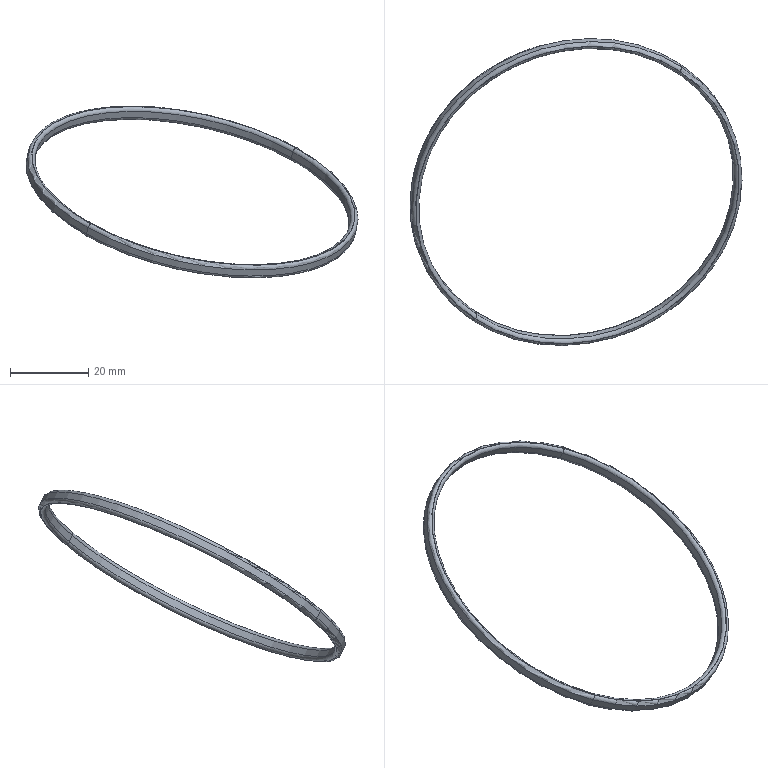Part | SolidWorks | features BaseBody 1 | 1 solid | 14 faces | box 84.752 x 78.463 x 43.87 mm | volume 1584 mm3 | torus 8 | cylinder 4 | plane 2 | commonest cylinder face diameters 82.4 x2 86.12 x2
STEP:
#1=CARTESIAN_POINT('',(1980.179,-187.025,950.905));
#2=VERTEX_POINT('',#1);
#3=CARTESIAN_POINT('',(1929.089,-248.825,931.919));
#4=VERTEX_POINT('',#3);
#5=CARTESIAN_POINT('',(1954.634,-217.925,941.412));
#6=DIRECTION('',(0.2015,-0.436,0.8771));
#7=DIRECTION('',(0.9077,0.4197,0.0001618));
#8=AXIS2_PLACEMENT_3D('',#5,#6,#7);
#9=CIRCLE('',#8,41.2);
#10=EDGE_CURVE('',#2,#4,#9,.T.);
#11=ORIENTED_EDGE('',*,*,#10,.F.);
#12=CARTESIAN_POINT('',(1980.539,-187.806,952.475));
#13=VERTEX_POINT('',#12);
#14=CARTESIAN_POINT('',(1980.359,-187.416,951.69));
#15=DIRECTION('',(0.2015,-0.436,0.8771));
#16=VECTOR('',#15,1000.);
#17=LINE('',#14,#16);
#18=EDGE_CURVE('',#2,#13,#17,.T.);
#19=ORIENTED_EDGE('',*,*,#18,.T.);
#20=CARTESIAN_POINT('',(1929.45,-249.605,933.489));
#21=VERTEX_POINT('',#20);
#22=CARTESIAN_POINT('',(1954.995,-218.706,942.982));
#23=DIRECTION('',(0.2015,-0.436,0.8771));
#24=DIRECTION('',(0.9077,0.4197,0.0001618));
#25=AXIS2_PLACEMENT_3D('',#22,#23,#24);
#26=CIRCLE('',#25,41.2);
#27=EDGE_CURVE('',#13,#21,#26,.T.);
#28=ORIENTED_EDGE('',*,*,#27,.T.);
#29=CARTESIAN_POINT('',(1929.27,-249.215,932.704));
#30=DIRECTION('',(-0.2015,0.436,-0.8771));
#31=VECTOR('',#30,1000.);
#32=LINE('',#29,#31);
#33=EDGE_CURVE('',#21,#4,#32,.T.);
#34=ORIENTED_EDGE('',*,*,#33,.T.);
#35=EDGE_LOOP('',(#11,#19,#28,#34));
#36=FACE_OUTER_BOUND('',#35,.T.);
#37=CARTESIAN_POINT('',(1954.814,-218.315,942.197));
#38=DIRECTION('',(0.2015,-0.436,0.8771));
#39=DIRECTION('',(-0.62,-0.75,-0.2304));
#40=AXIS2_PLACEMENT_3D('',#37,#38,#39);
#41=CYLINDRICAL_SURFACE('',#40,41.2);
#42=ADVANCED_FACE('',(#36),#41,.F.);
#43=CARTESIAN_POINT('',(1954.634,-217.925,941.412));
#44=DIRECTION('',(0.2015,-0.436,0.8771));
#45=DIRECTION('',(0.9077,0.4197,0.0001618));
#46=AXIS2_PLACEMENT_3D('',#43,#44,#45);
#47=CIRCLE('',#46,41.2);
#48=EDGE_CURVE('',#4,#2,#47,.T.);
#49=ORIENTED_EDGE('',*,*,#48,.F.);
#50=ORIENTED_EDGE('',*,*,#33,.F.);
#51=CARTESIAN_POINT('',(1954.995,-218.706,942.982));
#52=DIRECTION('',(0.2015,-0.436,0.8771));
#53=DIRECTION('',(0.9077,0.4197,0.0001618));
#54=AXIS2_PLACEMENT_3D('',#51,#52,#53);
#55=CIRCLE('',#54,41.2);
#56=EDGE_CURVE('',#21,#13,#55,.T.);
#57=ORIENTED_EDGE('',*,*,#56,.T.);
#58=ORIENTED_EDGE('',*,*,#18,.F.);
#59=EDGE_LOOP('',(#49,#50,#57,#58));
#60=FACE_OUTER_BOUND('',#59,.T.);
#61=CARTESIAN_POINT('',(1954.814,-218.315,942.197));
#62=DIRECTION('',(0.2015,-0.436,0.8771));
#63=DIRECTION('',(-0.62,-0.75,-0.2304));
#64=AXIS2_PLACEMENT_3D('',#61,#62,#63);
#65=CYLINDRICAL_SURFACE('',#64,41.2);
#66=ADVANCED_FACE('',(#60),#65,.F.);
#67=ORIENTED_EDGE('',*,*,#27,.F.);
#68=CARTESIAN_POINT('',(1981.279,-187.523,953.472));
#69=VERTEX_POINT('',#68);
#70=CARTESIAN_POINT('',(1981.097,-187.131,952.682));
#71=DIRECTION('',(0.7583,-0.4974,-0.4214));
#72=DIRECTION('',(0.62,0.75,0.2304));
#73=AXIS2_PLACEMENT_3D('',#70,#71,#72);
#74=CIRCLE('',#73,0.9);
#75=EDGE_CURVE('',#69,#13,#74,.T.);
#76=ORIENTED_EDGE('',*,*,#75,.F.);
#77=CARTESIAN_POINT('',(1929.073,-250.673,934.071));
#78=VERTEX_POINT('',#77);
#79=CARTESIAN_POINT('',(1955.176,-219.098,943.771));
#80=DIRECTION('',(0.2015,-0.436,0.8771));
#81=DIRECTION('',(0.9077,0.4197,0.0001618));
#82=AXIS2_PLACEMENT_3D('',#79,#80,#81);
#83=CIRCLE('',#82,42.1);
#84=EDGE_CURVE('',#69,#78,#83,.T.);
#85=ORIENTED_EDGE('',*,*,#84,.T.);
#86=CARTESIAN_POINT('',(1928.892,-250.28,933.281));
#87=DIRECTION('',(0.7583,-0.4974,-0.4214));
#88=DIRECTION('',(0.62,0.75,0.2304));
#89=AXIS2_PLACEMENT_3D('',#86,#87,#88);
#90=CIRCLE('',#89,0.9);
#91=EDGE_CURVE('',#21,#78,#90,.T.);
#92=ORIENTED_EDGE('',*,*,#91,.F.);
#93=EDGE_LOOP('',(#67,#76,#85,#92));
#94=FACE_OUTER_BOUND('',#93,.T.);
#95=CARTESIAN_POINT('',(1954.995,-218.706,942.982));
#96=DIRECTION('',(0.2015,-0.436,0.8771));
#97=DIRECTION('',(-0.62,-0.75,-0.2304));
#98=AXIS2_PLACEMENT_3D('',#95,#96,#97);
#99=TOROIDAL_SURFACE('',#98,42.1,0.9);
#100=ADVANCED_FACE('',(#94),#99,.T.);
#101=ORIENTED_EDGE('',*,*,#56,.F.);
#102=ORIENTED_EDGE('',*,*,#91,.T.);
#103=CARTESIAN_POINT('',(1955.176,-219.098,943.771));
#104=DIRECTION('',(0.2015,-0.436,0.8771));
#105=DIRECTION('',(0.9077,0.4197,0.0001618));
#106=AXIS2_PLACEMENT_3D('',#103,#104,#105);
#107=CIRCLE('',#106,42.1);
#108=EDGE_CURVE('',#78,#69,#107,.T.);
#109=ORIENTED_EDGE('',*,*,#108,.T.);
#110=ORIENTED_EDGE('',*,*,#75,.T.);
#111=EDGE_LOOP('',(#101,#102,#109,#110));
#112=FACE_OUTER_BOUND('',#111,.T.);
#113=CARTESIAN_POINT('',(1954.995,-218.706,942.982));
#114=DIRECTION('',(0.2015,-0.436,0.8771));
#115=DIRECTION('',(-0.62,-0.75,-0.2304));
#116=AXIS2_PLACEMENT_3D('',#113,#114,#115);
#117=TOROIDAL_SURFACE('',#116,42.1,0.9);
#118=ADVANCED_FACE('',(#112),#117,.T.);
#119=CARTESIAN_POINT('',(1981.316,-187.478,953.485));
#120=VERTEX_POINT('',#119);
#121=CARTESIAN_POINT('',(1929.036,-250.718,934.057));
#122=VERTEX_POINT('',#121);
#123=CARTESIAN_POINT('',(1955.176,-219.098,943.771));
#124=DIRECTION('',(0.2015,-0.436,0.8771));
#125=DIRECTION('',(0.9077,0.4197,0.0001618));
#126=AXIS2_PLACEMENT_3D('',#123,#124,#125);
#127=CIRCLE('',#126,42.16);
#128=EDGE_CURVE('',#120,#122,#127,.T.);
#129=ORIENTED_EDGE('',*,*,#128,.F.);
#130=CARTESIAN_POINT('',(1981.692,-186.411,952.903));
#131=VERTEX_POINT('',#130);
#132=CARTESIAN_POINT('',(1981.134,-187.086,952.696));
#133=DIRECTION('',(-0.7583,0.4974,0.4214));
#134=DIRECTION('',(0.62,0.75,0.2304));
#135=AXIS2_PLACEMENT_3D('',#132,#133,#134);
#136=CIRCLE('',#135,0.9);
#137=EDGE_CURVE('',#120,#131,#136,.T.);
#138=ORIENTED_EDGE('',*,*,#137,.T.);
#139=CARTESIAN_POINT('',(1928.297,-251.,933.06));
#140=VERTEX_POINT('',#139);
#141=CARTESIAN_POINT('',(1954.995,-218.706,942.982));
#142=DIRECTION('',(0.2015,-0.436,0.8771));
#143=DIRECTION('',(0.9077,0.4197,0.0001618));
#144=AXIS2_PLACEMENT_3D('',#141,#142,#143);
#145=CIRCLE('',#144,43.06);
#146=EDGE_CURVE('',#131,#140,#145,.T.);
#147=ORIENTED_EDGE('',*,*,#146,.T.);
#148=CARTESIAN_POINT('',(1928.855,-250.325,933.267));
#149=DIRECTION('',(-0.7583,0.4974,0.4214));
#150=DIRECTION('',(0.62,0.75,0.2304));
#151=AXIS2_PLACEMENT_3D('',#148,#149,#150);
#152=CIRCLE('',#151,0.9);
#153=EDGE_CURVE('',#140,#122,#152,.T.);
#154=ORIENTED_EDGE('',*,*,#153,.T.);
#155=EDGE_LOOP('',(#129,#138,#147,#154));
#156=FACE_OUTER_BOUND('',#155,.T.);
#157=CARTESIAN_POINT('',(1954.995,-218.706,942.982));
#158=DIRECTION('',(0.2015,-0.436,0.8771));
#159=DIRECTION('',(-0.62,-0.75,-0.2304));
#160=AXIS2_PLACEMENT_3D('',#157,#158,#159);
#161=TOROIDAL_SURFACE('',#160,42.16,0.9);
#162=ADVANCED_FACE('',(#156),#161,.T.);
#163=CARTESIAN_POINT('',(1955.176,-219.098,943.771));
#164=DIRECTION('',(0.2015,-0.436,0.8771));
#165=DIRECTION('',(0.9077,0.4197,0.0001618));
#166=AXIS2_PLACEMENT_3D('',#163,#164,#165);
#167=CIRCLE('',#166,42.16);
#168=EDGE_CURVE('',#122,#120,#167,.T.);
#169=ORIENTED_EDGE('',*,*,#168,.F.);
#170=ORIENTED_EDGE('',*,*,#153,.F.);
#171=CARTESIAN_POINT('',(1954.995,-218.706,942.982));
#172=DIRECTION('',(0.2015,-0.436,0.8771));
#173=DIRECTION('',(0.9077,0.4197,0.0001618));
#174=AXIS2_PLACEMENT_3D('',#171,#172,#173);
#175=CIRCLE('',#174,43.06);
#176=EDGE_CURVE('',#140,#131,#175,.T.);
#177=ORIENTED_EDGE('',*,*,#176,.T.);
#178=ORIENTED_EDGE('',*,*,#137,.F.);
#179=EDGE_LOOP('',(#169,#170,#177,#178));
#180=FACE_OUTER_BOUND('',#179,.T.);
#181=CARTESIAN_POINT('',(1954.995,-218.706,942.982));
#182=DIRECTION('',(0.2015,-0.436,0.8771));
#183=DIRECTION('',(-0.62,-0.75,-0.2304));
#184=AXIS2_PLACEMENT_3D('',#181,#182,#183);
#185=TOROIDAL_SURFACE('',#184,42.16,0.9);
#186=ADVANCED_FACE('',(#180),#185,.T.);
#187=ORIENTED_EDGE('',*,*,#146,.F.);
#188=CARTESIAN_POINT('',(1981.332,-185.63,951.333));
#189=VERTEX_POINT('',#188);
#190=CARTESIAN_POINT('',(1981.512,-186.021,952.118));
#191=DIRECTION('',(0.2015,-0.436,0.8771));
#192=VECTOR('',#191,1000.);
#193=LINE('',#190,#192);
#194=EDGE_CURVE('',#189,#131,#193,.T.);
#195=ORIENTED_EDGE('',*,*,#194,.F.);
#196=CARTESIAN_POINT('',(1927.936,-250.22,931.49));
#197=VERTEX_POINT('',#196);
#198=CARTESIAN_POINT('',(1954.634,-217.925,941.412));
#199=DIRECTION('',(0.2015,-0.436,0.8771));
#200=DIRECTION('',(0.9077,0.4197,0.0001618));
#201=AXIS2_PLACEMENT_3D('',#198,#199,#200);
#202=CIRCLE('',#201,43.06);
#203=EDGE_CURVE('',#189,#197,#202,.T.);
#204=ORIENTED_EDGE('',*,*,#203,.T.);
#205=CARTESIAN_POINT('',(1928.117,-250.61,932.275));
#206=DIRECTION('',(-0.2015,0.436,-0.8771));
#207=VECTOR('',#206,1000.);
#208=LINE('',#205,#207);
#209=EDGE_CURVE('',#140,#197,#208,.T.);
#210=ORIENTED_EDGE('',*,*,#209,.F.);
#211=EDGE_LOOP('',(#187,#195,#204,#210));
#212=FACE_OUTER_BOUND('',#211,.T.);
#213=CARTESIAN_POINT('',(1954.814,-218.315,942.197));
#214=DIRECTION('',(0.2015,-0.436,0.8771));
#215=DIRECTION('',(-0.62,-0.75,-0.2304));
#216=AXIS2_PLACEMENT_3D('',#213,#214,#215);
#217=CYLINDRICAL_SURFACE('',#216,43.06);
#218=ADVANCED_FACE('',(#212),#217,.T.);
#219=ORIENTED_EDGE('',*,*,#176,.F.);
#220=ORIENTED_EDGE('',*,*,#209,.T.);
#221=CARTESIAN_POINT('',(1954.634,-217.925,941.412));
#222=DIRECTION('',(0.2015,-0.436,0.8771));
#223=DIRECTION('',(0.9077,0.4197,0.0001618));
#224=AXIS2_PLACEMENT_3D('',#221,#222,#223);
#225=CIRCLE('',#224,43.06);
#226=EDGE_CURVE('',#197,#189,#225,.T.);
#227=ORIENTED_EDGE('',*,*,#226,.T.);
#228=ORIENTED_EDGE('',*,*,#194,.T.);
#229=EDGE_LOOP('',(#219,#220,#227,#228));
#230=FACE_OUTER_BOUND('',#229,.T.);
#231=CARTESIAN_POINT('',(1954.814,-218.315,942.197));
#232=DIRECTION('',(0.2015,-0.436,0.8771));
#233=DIRECTION('',(-0.62,-0.75,-0.2304));
#234=AXIS2_PLACEMENT_3D('',#231,#232,#233);
#235=CYLINDRICAL_SURFACE('',#234,43.06);
#236=ADVANCED_FACE('',(#230),#235,.T.);
#237=ORIENTED_EDGE('',*,*,#203,.F.);
#238=CARTESIAN_POINT('',(1980.592,-185.913,950.337));
#239=VERTEX_POINT('',#238);
#240=CARTESIAN_POINT('',(1980.774,-186.305,951.126));
#241=DIRECTION('',(0.7583,-0.4974,-0.4214));
#242=DIRECTION('',(0.62,0.75,0.2304));
#243=AXIS2_PLACEMENT_3D('',#240,#241,#242);
#244=CIRCLE('',#243,0.9);
#245=EDGE_CURVE('',#239,#189,#244,.T.);
#246=ORIENTED_EDGE('',*,*,#245,.F.);
#247=CARTESIAN_POINT('',(1928.313,-249.153,930.908));
#248=VERTEX_POINT('',#247);
#249=CARTESIAN_POINT('',(1954.453,-217.533,940.622));
#250=DIRECTION('',(0.2015,-0.436,0.8771));
#251=DIRECTION('',(0.9077,0.4197,0.0001618));
#252=AXIS2_PLACEMENT_3D('',#249,#250,#251);
#253=CIRCLE('',#252,42.16);
#254=EDGE_CURVE('',#239,#248,#253,.T.);
#255=ORIENTED_EDGE('',*,*,#254,.T.);
#256=CARTESIAN_POINT('',(1928.494,-249.545,931.697));
#257=DIRECTION('',(0.7583,-0.4974,-0.4214));
#258=DIRECTION('',(0.62,0.75,0.2304));
#259=AXIS2_PLACEMENT_3D('',#256,#257,#258);
#260=CIRCLE('',#259,0.9);
#261=EDGE_CURVE('',#197,#248,#260,.T.);
#262=ORIENTED_EDGE('',*,*,#261,.F.);
#263=EDGE_LOOP('',(#237,#246,#255,#262));
#264=FACE_OUTER_BOUND('',#263,.T.);
#265=CARTESIAN_POINT('',(1954.634,-217.925,941.412));
#266=DIRECTION('',(0.2015,-0.436,0.8771));
#267=DIRECTION('',(-0.62,-0.75,-0.2304));
#268=AXIS2_PLACEMENT_3D('',#265,#266,#267);
#269=TOROIDAL_SURFACE('',#268,42.16,0.9);
#270=ADVANCED_FACE('',(#264),#269,.T.);
#271=ORIENTED_EDGE('',*,*,#226,.F.);
#272=ORIENTED_EDGE('',*,*,#261,.T.);
#273=CARTESIAN_POINT('',(1954.453,-217.533,940.622));
#274=DIRECTION('',(0.2015,-0.436,0.8771));
#275=DIRECTION('',(0.9077,0.4197,0.0001618));
#276=AXIS2_PLACEMENT_3D('',#273,#274,#275);
#277=CIRCLE('',#276,42.16);
#278=EDGE_CURVE('',#248,#239,#277,.T.);
#279=ORIENTED_EDGE('',*,*,#278,.T.);
#280=ORIENTED_EDGE('',*,*,#245,.T.);
#281=EDGE_LOOP('',(#271,#272,#279,#280));
#282=FACE_OUTER_BOUND('',#281,.T.);
#283=CARTESIAN_POINT('',(1954.634,-217.925,941.412));
#284=DIRECTION('',(0.2015,-0.436,0.8771));
#285=DIRECTION('',(-0.62,-0.75,-0.2304));
#286=AXIS2_PLACEMENT_3D('',#283,#284,#285);
#287=TOROIDAL_SURFACE('',#286,42.16,0.9);
#288=ADVANCED_FACE('',(#282),#287,.T.);
#289=CARTESIAN_POINT('',(1980.555,-185.958,950.323));
#290=VERTEX_POINT('',#289);
#291=CARTESIAN_POINT('',(1928.35,-249.108,930.922));
#292=VERTEX_POINT('',#291);
#293=CARTESIAN_POINT('',(1954.453,-217.533,940.622));
#294=DIRECTION('',(0.2015,-0.436,0.8771));
#295=DIRECTION('',(0.9077,0.4197,0.0001618));
#296=AXIS2_PLACEMENT_3D('',#293,#294,#295);
#297=CIRCLE('',#296,42.1);
#298=EDGE_CURVE('',#290,#292,#297,.T.);
#299=ORIENTED_EDGE('',*,*,#298,.F.);
#300=CARTESIAN_POINT('',(1980.737,-186.35,951.112));
#301=DIRECTION('',(-0.7583,0.4974,0.4214));
#302=DIRECTION('',(0.62,0.75,0.2304));
#303=AXIS2_PLACEMENT_3D('',#300,#301,#302);
#304=CIRCLE('',#303,0.9);
#305=EDGE_CURVE('',#290,#2,#304,.T.);
#306=ORIENTED_EDGE('',*,*,#305,.T.);
#307=ORIENTED_EDGE('',*,*,#10,.T.);
#308=CARTESIAN_POINT('',(1928.531,-249.5,931.711));
#309=DIRECTION('',(-0.7583,0.4974,0.4214));
#310=DIRECTION('',(0.62,0.75,0.2304));
#311=AXIS2_PLACEMENT_3D('',#308,#309,#310);
#312=CIRCLE('',#311,0.9);
#313=EDGE_CURVE('',#4,#292,#312,.T.);
#314=ORIENTED_EDGE('',*,*,#313,.T.);
#315=EDGE_LOOP('',(#299,#306,#307,#314));
#316=FACE_OUTER_BOUND('',#315,.T.);
#317=CARTESIAN_POINT('',(1954.634,-217.925,941.412));
#318=DIRECTION('',(0.2015,-0.436,0.8771));
#319=DIRECTION('',(-0.62,-0.75,-0.2304));
#320=AXIS2_PLACEMENT_3D('',#317,#318,#319);
#321=TOROIDAL_SURFACE('',#320,42.1,0.9);
#322=ADVANCED_FACE('',(#316),#321,.T.);
#323=CARTESIAN_POINT('',(1954.453,-217.533,940.622));
#324=DIRECTION('',(0.2015,-0.436,0.8771));
#325=DIRECTION('',(0.9077,0.4197,0.0001618));
#326=AXIS2_PLACEMENT_3D('',#323,#324,#325);
#327=CIRCLE('',#326,42.1);
#328=EDGE_CURVE('',#292,#290,#327,.T.);
#329=ORIENTED_EDGE('',*,*,#328,.F.);
#330=ORIENTED_EDGE('',*,*,#313,.F.);
#331=ORIENTED_EDGE('',*,*,#48,.T.);
#332=ORIENTED_EDGE('',*,*,#305,.F.);
#333=EDGE_LOOP('',(#329,#330,#331,#332));
#334=FACE_OUTER_BOUND('',#333,.T.);
#335=CARTESIAN_POINT('',(1954.634,-217.925,941.412));
#336=DIRECTION('',(0.2015,-0.436,0.8771));
#337=DIRECTION('',(-0.62,-0.75,-0.2304));
#338=AXIS2_PLACEMENT_3D('',#335,#336,#337);
#339=TOROIDAL_SURFACE('',#338,42.1,0.9);
#340=ADVANCED_FACE('',(#334),#339,.T.);
#341=ORIENTED_EDGE('',*,*,#168,.T.);
#342=ORIENTED_EDGE('',*,*,#128,.T.);
#343=EDGE_LOOP('',(#341,#342));
#344=FACE_OUTER_BOUND('',#343,.T.);
#345=ORIENTED_EDGE('',*,*,#84,.F.);
#346=ORIENTED_EDGE('',*,*,#108,.F.);
#347=EDGE_LOOP('',(#345,#346));
#348=FACE_BOUND('',#347,.T.);
#349=CARTESIAN_POINT('',(1993.388,-201.428,943.778));
#350=DIRECTION('',(0.2015,-0.436,0.8771));
#351=DIRECTION('',(-0.9077,-0.4197,-0.0001618));
#352=AXIS2_PLACEMENT_3D('',#349,#350,#351);
#353=PLANE('',#352);
#354=ADVANCED_FACE('',(#344,#348),#353,.T.);
#355=ORIENTED_EDGE('',*,*,#254,.F.);
#356=ORIENTED_EDGE('',*,*,#278,.F.);
#357=EDGE_LOOP('',(#355,#356));
#358=FACE_OUTER_BOUND('',#357,.T.);
#359=ORIENTED_EDGE('',*,*,#328,.T.);
#360=ORIENTED_EDGE('',*,*,#298,.T.);
#361=EDGE_LOOP('',(#359,#360));
#362=FACE_BOUND('',#361,.T.);
#363=CARTESIAN_POINT('',(1992.719,-199.837,940.629));
#364=DIRECTION('',(0.2015,-0.436,0.8771));
#365=DIRECTION('',(-0.9077,-0.4197,-0.0001618));
#366=AXIS2_PLACEMENT_3D('',#363,#364,#365);
#367=PLANE('',#366);
#368=ADVANCED_FACE('',(#358,#362),#367,.F.);
#369=CLOSED_SHELL('',(#42,#66,#100,#118,#162,#186,#218,#236,#270,#288,#322,#340,#354,#368));
#370=MANIFOLD_SOLID_BREP('',#369);
#371=CARTESIAN_POINT('',(0.,0.,0.));
#372=DIRECTION('',(0.,0.,1.));
#373=DIRECTION('',(1.,0.,0.));
#374=AXIS2_PLACEMENT_3D('',#371,#372,#373);
#375=(LENGTH_UNIT()NAMED_UNIT(*)SI_UNIT(.MILLI.,.METRE.));
#376=UNCERTAINTY_MEASURE_WITH_UNIT(LENGTH_MEASURE(0.00001),#375,'','');
#377=(NAMED_UNIT(*)PLANE_ANGLE_UNIT()SI_UNIT($,.RADIAN.));
#378=(NAMED_UNIT(*)SI_UNIT($,.STERADIAN.)SOLID_ANGLE_UNIT());
#379=(GEOMETRIC_REPRESENTATION_CONTEXT(3)GLOBAL_UNCERTAINTY_ASSIGNED_CONTEXT((#376))GLOBAL_UNIT_ASSIGNED_CONTEXT((#375,#377,#378))REPRESENTATION_CONTEXT('',''));
#380=ADVANCED_BREP_SHAPE_REPRESENTATION('',(#370,#374),#379);